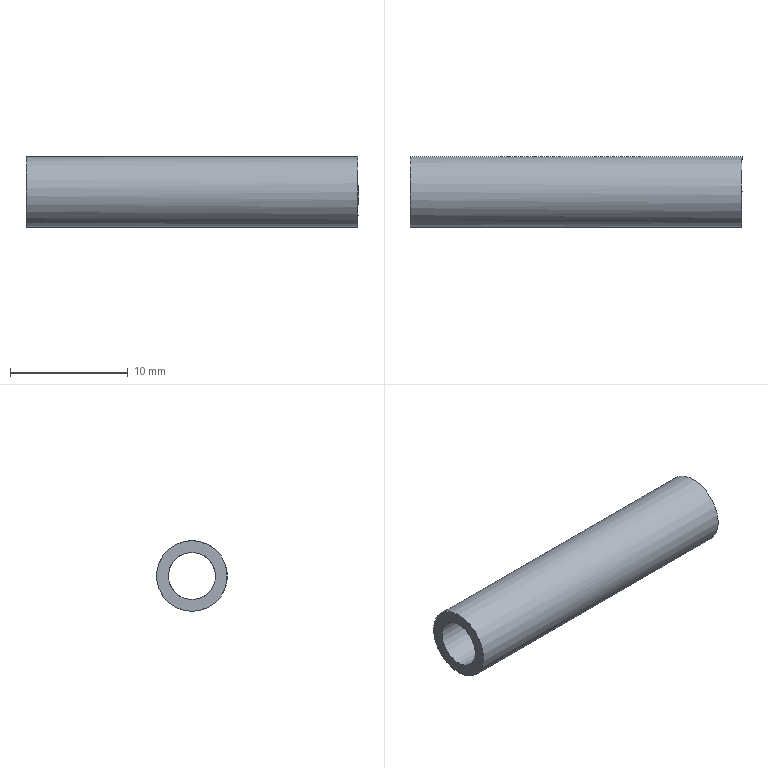Part | NX | features solid 2 | 1 solid | 4 faces | box 28.205 x 6 x 6 mm | volume 443.037 mm3 | cylinder 2 | plane 2 | commonest cylinder face diameters 4 x1 6 x1
STEP:
#1=CARTESIAN_POINT('',(-123.205,-109.,345.));
#2=VERTEX_POINT('',#1);
#3=CARTESIAN_POINT('',(-123.205,-109.,347.));
#4=DIRECTION('',(1.,0.,0.));
#5=DIRECTION('',(0.,0.,-1.));
#6=AXIS2_PLACEMENT_3D('',#3,#4,#5);
#7=CIRCLE('',#6,2.);
#8=EDGE_CURVE('',#2,#2,#7,.F.);
#9=ORIENTED_EDGE('',*,*,#8,.T.);
#10=EDGE_LOOP('',(#9));
#11=FACE_BOUND('',#10,.T.);
#12=CARTESIAN_POINT('',(-95.,-111.,347.));
#13=VERTEX_POINT('',#12);
#14=CARTESIAN_POINT('',(-95.,-109.,347.));
#15=DIRECTION('',(-1.,0.,0.));
#16=DIRECTION('',(0.,-1.,0.));
#17=AXIS2_PLACEMENT_3D('',#14,#15,#16);
#18=CIRCLE('',#17,2.);
#19=EDGE_CURVE('',#13,#13,#18,.T.);
#20=ORIENTED_EDGE('',*,*,#19,.F.);
#21=EDGE_LOOP('',(#20));
#22=FACE_BOUND('',#21,.T.);
#23=CARTESIAN_POINT('',(-273.824,-109.,347.));
#24=DIRECTION('',(1.,0.,0.));
#25=DIRECTION('',(0.,1.,0.));
#26=AXIS2_PLACEMENT_3D('',#23,#24,#25);
#27=CYLINDRICAL_SURFACE('',#26,2.);
#28=ADVANCED_FACE('',(#11,#22),#27,.F.);
#29=CARTESIAN_POINT('',(-123.205,-109.,344.));
#30=VERTEX_POINT('',#29);
#31=CARTESIAN_POINT('',(-123.205,-109.,347.));
#32=DIRECTION('',(1.,0.,0.));
#33=DIRECTION('',(0.,0.,-1.));
#34=AXIS2_PLACEMENT_3D('',#31,#32,#33);
#35=CIRCLE('',#34,3.);
#36=EDGE_CURVE('',#30,#30,#35,.F.);
#37=ORIENTED_EDGE('',*,*,#36,.F.);
#38=EDGE_LOOP('',(#37));
#39=FACE_BOUND('',#38,.T.);
#40=CARTESIAN_POINT('',(-95.,-112.,347.));
#41=VERTEX_POINT('',#40);
#42=CARTESIAN_POINT('',(-95.,-109.,347.));
#43=DIRECTION('',(-1.,0.,0.));
#44=DIRECTION('',(0.,-1.,0.));
#45=AXIS2_PLACEMENT_3D('',#42,#43,#44);
#46=CIRCLE('',#45,3.);
#47=EDGE_CURVE('',#41,#41,#46,.T.);
#48=ORIENTED_EDGE('',*,*,#47,.T.);
#49=EDGE_LOOP('',(#48));
#50=FACE_BOUND('',#49,.T.);
#51=CARTESIAN_POINT('',(-273.824,-109.,347.));
#52=DIRECTION('',(1.,0.,0.));
#53=DIRECTION('',(0.,1.,0.));
#54=AXIS2_PLACEMENT_3D('',#51,#52,#53);
#55=CYLINDRICAL_SURFACE('',#54,3.);
#56=ADVANCED_FACE('',(#39,#50),#55,.T.);
#57=ORIENTED_EDGE('',*,*,#8,.F.);
#58=EDGE_LOOP('',(#57));
#59=FACE_BOUND('',#58,.T.);
#60=ORIENTED_EDGE('',*,*,#36,.T.);
#61=EDGE_LOOP('',(#60));
#62=FACE_BOUND('',#61,.T.);
#63=CARTESIAN_POINT('',(-123.205,-140.535,126.));
#64=DIRECTION('',(1.,0.,0.));
#65=DIRECTION('',(0.,1.,0.));
#66=AXIS2_PLACEMENT_3D('',#63,#64,#65);
#67=PLANE('',#66);
#68=ADVANCED_FACE('',(#59,#62),#67,.F.);
#69=ORIENTED_EDGE('',*,*,#19,.T.);
#70=EDGE_LOOP('',(#69));
#71=FACE_BOUND('',#70,.T.);
#72=ORIENTED_EDGE('',*,*,#47,.F.);
#73=EDGE_LOOP('',(#72));
#74=FACE_BOUND('',#73,.T.);
#75=CARTESIAN_POINT('',(-95.,-109.,347.));
#76=DIRECTION('',(-1.,0.,0.));
#77=DIRECTION('',(0.,-1.,0.));
#78=AXIS2_PLACEMENT_3D('',#75,#76,#77);
#79=PLANE('',#78);
#80=ADVANCED_FACE('',(#71,#74),#79,.F.);
#81=CLOSED_SHELL('',(#28,#56,#68,#80));
#82=MANIFOLD_SOLID_BREP('',#81);
#83=(LENGTH_UNIT()NAMED_UNIT(*)SI_UNIT(.MILLI.,.METRE.));
#84=UNCERTAINTY_MEASURE_WITH_UNIT(LENGTH_MEASURE(0.00001),#83,'','');
#85=(NAMED_UNIT(*)PLANE_ANGLE_UNIT()SI_UNIT($,.RADIAN.));
#86=(NAMED_UNIT(*)SI_UNIT($,.STERADIAN.)SOLID_ANGLE_UNIT());
#87=(GEOMETRIC_REPRESENTATION_CONTEXT(3)GLOBAL_UNCERTAINTY_ASSIGNED_CONTEXT((#84))GLOBAL_UNIT_ASSIGNED_CONTEXT((#83,#85,#86))REPRESENTATION_CONTEXT('',''));
#88=ADVANCED_BREP_SHAPE_REPRESENTATION('',(#82),#87);